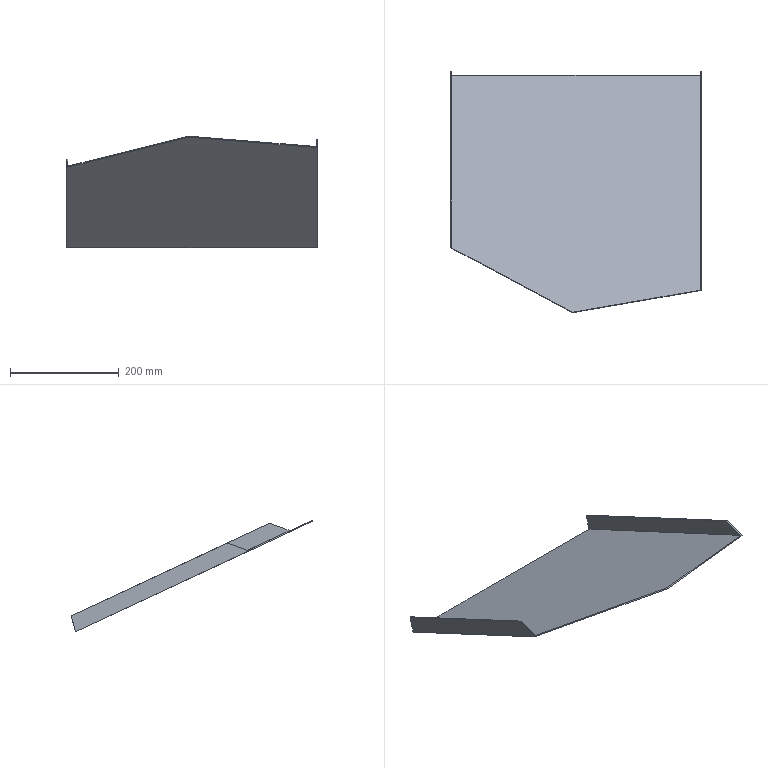Part | NX | features solid 2 | 1 solid | 13 faces | box 459.123 x 443.36 x 204.878 mm | volume 442508 mm3 | plane 12 | spline 1
STEP:
#1=CARTESIAN_POINT('',(40.63,399.571,-277.28));
#2=VERTEX_POINT('',#1);
#3=CARTESIAN_POINT('',(40.63,793.782,-461.104));
#4=VERTEX_POINT('',#3);
#5=CARTESIAN_POINT('',(40.63,358.626,-258.187));
#6=DIRECTION('',(0.,0.9063,-0.4226));
#7=VECTOR('',#6,1000.);
#8=LINE('',#5,#7);
#9=EDGE_CURVE('',#2,#4,#8,.T.);
#10=ORIENTED_EDGE('',*,*,#9,.T.);
#11=CARTESIAN_POINT('',(-414.493,793.782,-461.104));
#12=VERTEX_POINT('',#11);
#13=CARTESIAN_POINT('',(-192.912,793.782,-461.104));
#14=DIRECTION('',(-1.,0.,0.));
#15=VECTOR('',#14,1000.);
#16=LINE('',#13,#15);
#17=EDGE_CURVE('',#4,#12,#16,.T.);
#18=ORIENTED_EDGE('',*,*,#17,.T.);
#19=CARTESIAN_POINT('',(-414.493,477.671,-313.699));
#20=VERTEX_POINT('',#19);
#21=CARTESIAN_POINT('',(-414.493,358.626,-258.187));
#22=DIRECTION('',(0.,0.9063,-0.4226));
#23=VECTOR('',#22,1000.);
#24=LINE('',#21,#23);
#25=EDGE_CURVE('',#20,#12,#24,.T.);
#26=ORIENTED_EDGE('',*,*,#25,.F.);
#27=CARTESIAN_POINT('',(-416.493,477.671,-313.699));
#28=VERTEX_POINT('',#27);
#29=CARTESIAN_POINT('',(-416.493,477.671,-313.699));
#30=DIRECTION('',(-1.,0.,0.));
#31=VECTOR('',#30,1000.);
#32=LINE('',#29,#31);
#33=EDGE_CURVE('',#20,#28,#32,.T.);
#34=ORIENTED_EDGE('',*,*,#33,.T.);
#35=CARTESIAN_POINT('',(-192.912,358.626,-258.187));
#36=VERTEX_POINT('',#35);
#37=CARTESIAN_POINT('',(-192.912,358.626,-258.187));
#38=DIRECTION('',(0.8622,-0.4591,0.2141));
#39=VECTOR('',#38,1000.);
#40=LINE('',#37,#39);
#41=EDGE_CURVE('',#28,#36,#40,.T.);
#42=ORIENTED_EDGE('',*,*,#41,.T.);
#43=CARTESIAN_POINT('',(42.63,399.571,-277.28));
#44=VERTEX_POINT('',#43);
#45=CARTESIAN_POINT('',(-192.912,358.626,-258.187));
#46=CARTESIAN_POINT('',(-183.102,360.356,-258.994));
#47=CARTESIAN_POINT('',(-163.484,363.815,-260.607));
#48=CARTESIAN_POINT('',(-134.056,369.003,-263.026));
#49=CARTESIAN_POINT('',(-104.626,374.192,-265.446));
#50=CARTESIAN_POINT('',(-80.109,378.513,-267.461));
#51=CARTESIAN_POINT('',(-62.932,381.543,-268.874));
#52=CARTESIAN_POINT('',(-53.141,383.273,-269.68));
#53=CARTESIAN_POINT('',(-45.731,384.584,-270.292));
#54=CARTESIAN_POINT('',(-38.576,385.847,-270.88));
#55=CARTESIAN_POINT('',(-31.239,387.132,-271.48));
#56=CARTESIAN_POINT('',(-25.081,388.204,-271.98));
#57=CARTESIAN_POINT('',(-20.086,389.069,-272.383));
#58=CARTESIAN_POINT('',(-16.374,389.711,-272.682));
#59=CARTESIAN_POINT('',(-12.429,390.39,-272.999));
#60=CARTESIAN_POINT('',(-8.618,391.042,-273.303));
#61=CARTESIAN_POINT('',(-4.844,391.685,-273.603));
#62=CARTESIAN_POINT('',(-1.133,392.314,-273.896));
#63=CARTESIAN_POINT('',(2.523,392.93,-274.184));
#64=CARTESIAN_POINT('',(5.521,393.433,-274.418));
#65=CARTESIAN_POINT('',(7.891,393.829,-274.602));
#66=CARTESIAN_POINT('',(9.657,394.123,-274.74));
#67=CARTESIAN_POINT('',(11.104,394.363,-274.852));
#68=CARTESIAN_POINT('',(12.137,394.534,-274.931));
#69=CARTESIAN_POINT('',(12.684,394.624,-274.973));
#70=CARTESIAN_POINT('',(13.211,394.711,-275.014));
#71=CARTESIAN_POINT('',(13.289,394.724,-275.02));
#72=CARTESIAN_POINT('',(13.565,394.77,-275.041));
#73=CARTESIAN_POINT('',(14.006,394.843,-275.075));
#74=CARTESIAN_POINT('',(14.766,394.968,-275.134));
#75=CARTESIAN_POINT('',(15.806,395.14,-275.214));
#76=CARTESIAN_POINT('',(17.393,395.402,-275.336));
#77=CARTESIAN_POINT('',(19.737,395.789,-275.517));
#78=CARTESIAN_POINT('',(23.133,396.35,-275.778));
#79=CARTESIAN_POINT('',(27.111,397.007,-276.085));
#80=CARTESIAN_POINT('',(33.19,398.012,-276.553));
#81=CARTESIAN_POINT('',(38.621,398.909,-276.971));
#82=CARTESIAN_POINT('',(42.63,399.571,-277.28));
#83=B_SPLINE_CURVE_WITH_KNOTS('',3,(#45,#46,#47,#48,#49,#50,#51,#52,#53,#54,#55,#56,#57,#58,#59,#60,#61,#62,#63,#64,#65,#66,#67,#68,#69,#70,#71,#72,#73,#74,#75,#76,#77,#78,#79,#80,#81,#82),.UNSPECIFIED.,.F.,.F.,(4,1,1,1,1,1,1,1,1,1,1,1,1,1,1,1,1,1,1,1,1,1,1,1,1,1,1,1,1,1,1,1,1,1,1,4),(0.,0.125,0.25,0.375,0.5,0.5625,0.5938,0.625,0.6562,0.6875,0.7188,0.7344,0.75,0.7656,0.7812,0.7969,0.8125,0.8281,0.8438,0.8516,0.8594,0.8672,0.8711,0.873,0.875,0.877,0.8789,0.8828,0.8906,0.8984,0.9062,0.9219,0.9375,0.9531,0.9688,1.),.UNSPECIFIED.);
#84=EDGE_CURVE('',#44,#36,#83,.F.);
#85=ORIENTED_EDGE('',*,*,#84,.F.);
#86=CARTESIAN_POINT('',(42.63,399.571,-277.28));
#87=DIRECTION('',(1.,0.,0.));
#88=VECTOR('',#87,1000.);
#89=LINE('',#86,#88);
#90=EDGE_CURVE('',#44,#2,#89,.F.);
#91=ORIENTED_EDGE('',*,*,#90,.T.);
#92=EDGE_LOOP('',(#10,#18,#26,#34,#42,#85,#91));
#93=FACE_BOUND('',#92,.T.);
#94=CARTESIAN_POINT('',(-192.912,358.626,-258.187));
#95=DIRECTION('',(0.,-0.4226,-0.9063));
#96=DIRECTION('',(-1.,0.,0.));
#97=AXIS2_PLACEMENT_3D('',#94,#95,#96);
#98=PLANE('',#97);
#99=ADVANCED_FACE('',(#93),#98,.F.);
#100=ORIENTED_EDGE('',*,*,#84,.T.);
#101=CARTESIAN_POINT('',(-192.912,357.781,-260.));
#102=VERTEX_POINT('',#101);
#103=CARTESIAN_POINT('',(-192.912,358.626,-258.187));
#104=CARTESIAN_POINT('',(-192.912,358.345,-258.792));
#105=CARTESIAN_POINT('',(-192.912,358.063,-259.396));
#106=CARTESIAN_POINT('',(-192.912,357.781,-260.));
#107=B_SPLINE_CURVE_WITH_KNOTS('',3,(#103,#104,#105,#106),.UNSPECIFIED.,.F.,.F.,(4,4),(0.,1.),.UNSPECIFIED.);
#108=EDGE_CURVE('',#102,#36,#107,.F.);
#109=ORIENTED_EDGE('',*,*,#108,.F.);
#110=CARTESIAN_POINT('',(42.63,398.726,-279.093));
#111=VERTEX_POINT('',#110);
#112=CARTESIAN_POINT('',(-192.912,357.781,-260.));
#113=CARTESIAN_POINT('',(-183.102,359.511,-260.807));
#114=CARTESIAN_POINT('',(-163.484,362.97,-262.42));
#115=CARTESIAN_POINT('',(-134.056,368.158,-264.839));
#116=CARTESIAN_POINT('',(-104.626,373.347,-267.258));
#117=CARTESIAN_POINT('',(-80.109,377.668,-269.273));
#118=CARTESIAN_POINT('',(-62.932,380.698,-270.686));
#119=CARTESIAN_POINT('',(-53.141,382.427,-271.493));
#120=CARTESIAN_POINT('',(-45.731,383.739,-272.104));
#121=CARTESIAN_POINT('',(-38.576,385.001,-272.693));
#122=CARTESIAN_POINT('',(-31.239,386.287,-273.292));
#123=CARTESIAN_POINT('',(-25.081,387.359,-273.792));
#124=CARTESIAN_POINT('',(-20.086,388.224,-274.196));
#125=CARTESIAN_POINT('',(-16.374,388.865,-274.495));
#126=CARTESIAN_POINT('',(-12.429,389.544,-274.811));
#127=CARTESIAN_POINT('',(-8.618,390.197,-275.116));
#128=CARTESIAN_POINT('',(-4.844,390.84,-275.415));
#129=CARTESIAN_POINT('',(-1.133,391.469,-275.709));
#130=CARTESIAN_POINT('',(2.523,392.085,-275.996));
#131=CARTESIAN_POINT('',(5.521,392.588,-276.231));
#132=CARTESIAN_POINT('',(7.891,392.983,-276.415));
#133=CARTESIAN_POINT('',(9.657,393.277,-276.552));
#134=CARTESIAN_POINT('',(11.104,393.518,-276.664));
#135=CARTESIAN_POINT('',(12.137,393.689,-276.744));
#136=CARTESIAN_POINT('',(12.684,393.779,-276.786));
#137=CARTESIAN_POINT('',(13.211,393.866,-276.827));
#138=CARTESIAN_POINT('',(13.289,393.879,-276.833));
#139=CARTESIAN_POINT('',(13.565,393.925,-276.854));
#140=CARTESIAN_POINT('',(14.006,393.997,-276.888));
#141=CARTESIAN_POINT('',(14.766,394.123,-276.946));
#142=CARTESIAN_POINT('',(15.806,394.295,-277.027));
#143=CARTESIAN_POINT('',(17.393,394.557,-277.149));
#144=CARTESIAN_POINT('',(19.737,394.944,-277.329));
#145=CARTESIAN_POINT('',(23.133,395.505,-277.591));
#146=CARTESIAN_POINT('',(27.111,396.162,-277.897));
#147=CARTESIAN_POINT('',(33.19,397.166,-278.366));
#148=CARTESIAN_POINT('',(38.621,398.064,-278.784));
#149=CARTESIAN_POINT('',(42.63,398.726,-279.093));
#150=B_SPLINE_CURVE_WITH_KNOTS('',3,(#112,#113,#114,#115,#116,#117,#118,#119,#120,#121,#122,#123,#124,#125,#126,#127,#128,#129,#130,#131,#132,#133,#134,#135,#136,#137,#138,#139,#140,#141,#142,#143,#144,#145,#146,#147,#148,#149),.UNSPECIFIED.,.F.,.F.,(4,1,1,1,1,1,1,1,1,1,1,1,1,1,1,1,1,1,1,1,1,1,1,1,1,1,1,1,1,1,1,1,1,1,1,4),(0.,0.125,0.25,0.375,0.5,0.5625,0.5938,0.625,0.6562,0.6875,0.7188,0.7344,0.75,0.7656,0.7812,0.7969,0.8125,0.8281,0.8438,0.8516,0.8594,0.8672,0.8711,0.873,0.875,0.877,0.8789,0.8828,0.8906,0.8984,0.9062,0.9219,0.9375,0.9531,0.9688,1.),.UNSPECIFIED.);
#151=EDGE_CURVE('',#111,#102,#150,.F.);
#152=ORIENTED_EDGE('',*,*,#151,.F.);
#153=CARTESIAN_POINT('',(42.63,398.726,-279.093));
#154=CARTESIAN_POINT('',(42.63,399.008,-278.489));
#155=CARTESIAN_POINT('',(42.63,399.289,-277.884));
#156=CARTESIAN_POINT('',(42.63,399.571,-277.28));
#157=B_SPLINE_CURVE_WITH_KNOTS('',3,(#153,#154,#155,#156),.UNSPECIFIED.,.F.,.F.,(4,4),(0.,1.),.UNSPECIFIED.);
#158=EDGE_CURVE('',#111,#44,#157,.T.);
#159=ORIENTED_EDGE('',*,*,#158,.T.);
#160=EDGE_LOOP('',(#100,#109,#152,#159));
#161=FACE_BOUND('',#160,.T.);
#162=CARTESIAN_POINT('',(-192.912,357.781,-260.));
#163=CARTESIAN_POINT('',(-192.912,358.626,-258.187));
#164=CARTESIAN_POINT('',(-183.102,359.511,-260.807));
#165=CARTESIAN_POINT('',(-183.102,360.356,-258.994));
#166=CARTESIAN_POINT('',(-163.484,362.97,-262.42));
#167=CARTESIAN_POINT('',(-163.484,363.815,-260.607));
#168=CARTESIAN_POINT('',(-134.056,368.158,-264.839));
#169=CARTESIAN_POINT('',(-134.056,369.003,-263.026));
#170=CARTESIAN_POINT('',(-104.626,373.347,-267.258));
#171=CARTESIAN_POINT('',(-104.626,374.192,-265.446));
#172=CARTESIAN_POINT('',(-80.109,377.668,-269.273));
#173=CARTESIAN_POINT('',(-80.109,378.513,-267.461));
#174=CARTESIAN_POINT('',(-62.932,380.698,-270.686));
#175=CARTESIAN_POINT('',(-62.932,381.543,-268.874));
#176=CARTESIAN_POINT('',(-53.141,382.427,-271.493));
#177=CARTESIAN_POINT('',(-53.141,383.273,-269.68));
#178=CARTESIAN_POINT('',(-45.731,383.739,-272.104));
#179=CARTESIAN_POINT('',(-45.731,384.584,-270.292));
#180=CARTESIAN_POINT('',(-38.576,385.001,-272.693));
#181=CARTESIAN_POINT('',(-38.576,385.847,-270.88));
#182=CARTESIAN_POINT('',(-31.239,386.287,-273.292));
#183=CARTESIAN_POINT('',(-31.239,387.132,-271.48));
#184=CARTESIAN_POINT('',(-25.081,387.359,-273.792));
#185=CARTESIAN_POINT('',(-25.081,388.204,-271.98));
#186=CARTESIAN_POINT('',(-20.086,388.224,-274.196));
#187=CARTESIAN_POINT('',(-20.086,389.069,-272.383));
#188=CARTESIAN_POINT('',(-16.374,388.865,-274.495));
#189=CARTESIAN_POINT('',(-16.374,389.711,-272.682));
#190=CARTESIAN_POINT('',(-12.429,389.544,-274.811));
#191=CARTESIAN_POINT('',(-12.429,390.39,-272.999));
#192=CARTESIAN_POINT('',(-8.618,390.197,-275.116));
#193=CARTESIAN_POINT('',(-8.618,391.042,-273.303));
#194=CARTESIAN_POINT('',(-4.844,390.84,-275.415));
#195=CARTESIAN_POINT('',(-4.844,391.685,-273.603));
#196=CARTESIAN_POINT('',(-1.133,391.469,-275.709));
#197=CARTESIAN_POINT('',(-1.133,392.314,-273.896));
#198=CARTESIAN_POINT('',(2.523,392.085,-275.996));
#199=CARTESIAN_POINT('',(2.523,392.93,-274.184));
#200=CARTESIAN_POINT('',(5.521,392.588,-276.231));
#201=CARTESIAN_POINT('',(5.521,393.433,-274.418));
#202=CARTESIAN_POINT('',(7.891,392.983,-276.415));
#203=CARTESIAN_POINT('',(7.891,393.829,-274.602));
#204=CARTESIAN_POINT('',(9.657,393.277,-276.552));
#205=CARTESIAN_POINT('',(9.657,394.123,-274.74));
#206=CARTESIAN_POINT('',(11.104,393.518,-276.664));
#207=CARTESIAN_POINT('',(11.104,394.363,-274.852));
#208=CARTESIAN_POINT('',(12.137,393.689,-276.744));
#209=CARTESIAN_POINT('',(12.137,394.534,-274.931));
#210=CARTESIAN_POINT('',(12.684,393.779,-276.786));
#211=CARTESIAN_POINT('',(12.684,394.624,-274.973));
#212=CARTESIAN_POINT('',(13.211,393.866,-276.827));
#213=CARTESIAN_POINT('',(13.211,394.711,-275.014));
#214=CARTESIAN_POINT('',(13.289,393.879,-276.833));
#215=CARTESIAN_POINT('',(13.289,394.724,-275.02));
#216=CARTESIAN_POINT('',(13.565,393.925,-276.854));
#217=CARTESIAN_POINT('',(13.565,394.77,-275.041));
#218=CARTESIAN_POINT('',(14.006,393.997,-276.888));
#219=CARTESIAN_POINT('',(14.006,394.843,-275.075));
#220=CARTESIAN_POINT('',(14.766,394.123,-276.946));
#221=CARTESIAN_POINT('',(14.766,394.968,-275.134));
#222=CARTESIAN_POINT('',(15.806,394.295,-277.027));
#223=CARTESIAN_POINT('',(15.806,395.14,-275.214));
#224=CARTESIAN_POINT('',(17.393,394.557,-277.149));
#225=CARTESIAN_POINT('',(17.393,395.402,-275.336));
#226=CARTESIAN_POINT('',(19.737,394.944,-277.329));
#227=CARTESIAN_POINT('',(19.737,395.789,-275.517));
#228=CARTESIAN_POINT('',(23.133,395.505,-277.591));
#229=CARTESIAN_POINT('',(23.133,396.35,-275.778));
#230=CARTESIAN_POINT('',(27.111,396.162,-277.897));
#231=CARTESIAN_POINT('',(27.111,397.007,-276.085));
#232=CARTESIAN_POINT('',(33.19,397.166,-278.366));
#233=CARTESIAN_POINT('',(33.19,398.012,-276.553));
#234=CARTESIAN_POINT('',(38.621,398.064,-278.784));
#235=CARTESIAN_POINT('',(38.621,398.909,-276.971));
#236=CARTESIAN_POINT('',(42.63,398.726,-279.093));
#237=CARTESIAN_POINT('',(42.63,399.571,-277.28));
#238=B_SPLINE_SURFACE_WITH_KNOTS('',3,1,((#162,#163),(#164,#165),(#166,#167),(#168,#169),(#170,#171),(#172,#173),(#174,#175),(#176,#177),(#178,#179),(#180,#181),(#182,#183),(#184,#185),(#186,#187),(#188,#189),(#190,#191),(#192,#193),(#194,#195),(#196,#197),(#198,#199),(#200,#201),(#202,#203),(#204,#205),(#206,#207),(#208,#209),(#210,#211),(#212,#213),(#214,#215),(#216,#217),(#218,#219),(#220,#221),(#222,#223),(#224,#225),(#226,#227),(#228,#229),(#230,#231),(#232,#233),(#234,#235),(#236,#237)),.SURF_OF_LINEAR_EXTRUSION.,.F.,.F.,.F.,(4,1,1,1,1,1,1,1,1,1,1,1,1,1,1,1,1,1,1,1,1,1,1,1,1,1,1,1,1,1,1,1,1,1,1,4),(2,2),(0.,0.125,0.25,0.375,0.5,0.5625,0.5938,0.625,0.6562,0.6875,0.7188,0.7344,0.75,0.7656,0.7812,0.7969,0.8125,0.8281,0.8438,0.8516,0.8594,0.8672,0.8711,0.873,0.875,0.877,0.8789,0.8828,0.8906,0.8984,0.9062,0.9219,0.9375,0.9531,0.9688,1.),(0.,1.),.UNSPECIFIED.);
#239=ADVANCED_FACE('',(#161),#238,.T.);
#240=CARTESIAN_POINT('',(42.63,793.257,-463.066));
#241=VERTEX_POINT('',#240);
#242=CARTESIAN_POINT('',(42.63,357.781,-260.));
#243=DIRECTION('',(0.,-0.9063,0.4226));
#244=VECTOR('',#243,1000.);
#245=LINE('',#242,#244);
#246=EDGE_CURVE('',#241,#111,#245,.T.);
#247=ORIENTED_EDGE('',*,*,#246,.F.);
#248=CARTESIAN_POINT('',(42.63,801.141,-433.641));
#249=VERTEX_POINT('',#248);
#250=CARTESIAN_POINT('',(42.63,814.852,-382.472));
#251=DIRECTION('',(0.,0.2588,0.9659));
#252=VECTOR('',#251,1000.);
#253=LINE('',#250,#252);
#254=EDGE_CURVE('',#241,#249,#253,.T.);
#255=ORIENTED_EDGE('',*,*,#254,.T.);
#256=CARTESIAN_POINT('',(42.63,436.781,-263.737));
#257=VERTEX_POINT('',#256);
#258=CARTESIAN_POINT('',(42.63,1052.679,-550.935));
#259=DIRECTION('',(0.,-0.9063,0.4226));
#260=VECTOR('',#259,1000.);
#261=LINE('',#258,#260);
#262=EDGE_CURVE('',#249,#257,#261,.T.);
#263=ORIENTED_EDGE('',*,*,#262,.T.);
#264=CARTESIAN_POINT('',(42.63,399.571,-277.28));
#265=DIRECTION('',(0.,-0.9397,-0.342));
#266=VECTOR('',#265,1000.);
#267=LINE('',#264,#266);
#268=EDGE_CURVE('',#257,#44,#267,.T.);
#269=ORIENTED_EDGE('',*,*,#268,.T.);
#270=ORIENTED_EDGE('',*,*,#158,.F.);
#271=EDGE_LOOP('',(#247,#255,#263,#269,#270));
#272=FACE_BOUND('',#271,.T.);
#273=CARTESIAN_POINT('',(42.63,357.781,-260.));
#274=DIRECTION('',(-1.,0.,0.));
#275=DIRECTION('',(0.,0.,1.));
#276=AXIS2_PLACEMENT_3D('',#273,#274,#275);
#277=PLANE('',#276);
#278=ADVANCED_FACE('',(#272),#277,.F.);
#279=CARTESIAN_POINT('',(-416.493,793.257,-463.066));
#280=VERTEX_POINT('',#279);
#281=CARTESIAN_POINT('',(-416.493,801.141,-433.641));
#282=VERTEX_POINT('',#281);
#283=CARTESIAN_POINT('',(-416.493,814.852,-382.472));
#284=DIRECTION('',(0.,0.2588,0.9659));
#285=VECTOR('',#284,1000.);
#286=LINE('',#283,#285);
#287=EDGE_CURVE('',#280,#282,#286,.T.);
#288=ORIENTED_EDGE('',*,*,#287,.F.);
#289=CARTESIAN_POINT('',(-416.493,476.826,-315.512));
#290=VERTEX_POINT('',#289);
#291=CARTESIAN_POINT('',(-416.493,357.781,-260.));
#292=DIRECTION('',(0.,-0.9063,0.4226));
#293=VECTOR('',#292,1000.);
#294=LINE('',#291,#293);
#295=EDGE_CURVE('',#280,#290,#294,.T.);
#296=ORIENTED_EDGE('',*,*,#295,.T.);
#297=CARTESIAN_POINT('',(-416.493,476.826,-315.512));
#298=DIRECTION('',(0.,0.4226,0.9063));
#299=VECTOR('',#298,1000.);
#300=LINE('',#297,#299);
#301=EDGE_CURVE('',#290,#28,#300,.T.);
#302=ORIENTED_EDGE('',*,*,#301,.T.);
#303=CARTESIAN_POINT('',(-416.493,514.881,-300.156));
#304=VERTEX_POINT('',#303);
#305=CARTESIAN_POINT('',(-416.493,889.235,-163.902));
#306=DIRECTION('',(0.,0.9397,0.342));
#307=VECTOR('',#306,1000.);
#308=LINE('',#305,#307);
#309=EDGE_CURVE('',#28,#304,#308,.T.);
#310=ORIENTED_EDGE('',*,*,#309,.T.);
#311=CARTESIAN_POINT('',(-416.493,1052.679,-550.935));
#312=DIRECTION('',(0.,-0.9063,0.4226));
#313=VECTOR('',#312,1000.);
#314=LINE('',#311,#313);
#315=EDGE_CURVE('',#282,#304,#314,.T.);
#316=ORIENTED_EDGE('',*,*,#315,.F.);
#317=EDGE_LOOP('',(#288,#296,#302,#310,#316));
#318=FACE_BOUND('',#317,.T.);
#319=CARTESIAN_POINT('',(-416.493,357.781,-260.));
#320=DIRECTION('',(-1.,0.,0.));
#321=DIRECTION('',(0.,0.,1.));
#322=AXIS2_PLACEMENT_3D('',#319,#320,#321);
#323=PLANE('',#322);
#324=ADVANCED_FACE('',(#318),#323,.T.);
#325=ORIENTED_EDGE('',*,*,#41,.F.);
#326=ORIENTED_EDGE('',*,*,#301,.F.);
#327=CARTESIAN_POINT('',(-192.912,357.781,-260.));
#328=DIRECTION('',(0.8622,-0.4591,0.2141));
#329=VECTOR('',#328,1000.);
#330=LINE('',#327,#329);
#331=EDGE_CURVE('',#290,#102,#330,.T.);
#332=ORIENTED_EDGE('',*,*,#331,.T.);
#333=ORIENTED_EDGE('',*,*,#108,.T.);
#334=EDGE_LOOP('',(#325,#326,#332,#333));
#335=FACE_BOUND('',#334,.T.);
#336=CARTESIAN_POINT('',(-192.912,357.781,-260.));
#337=DIRECTION('',(-0.5065,-0.7814,0.3644));
#338=DIRECTION('',(0.8391,-0.5439,0.));
#339=AXIS2_PLACEMENT_3D('',#336,#337,#338);
#340=PLANE('',#339);
#341=ADVANCED_FACE('',(#335),#340,.T.);
#342=CARTESIAN_POINT('',(-192.912,793.257,-463.066));
#343=DIRECTION('',(-1.,0.,0.));
#344=VECTOR('',#343,1000.);
#345=LINE('',#342,#344);
#346=EDGE_CURVE('',#241,#280,#345,.T.);
#347=ORIENTED_EDGE('',*,*,#346,.F.);
#348=ORIENTED_EDGE('',*,*,#246,.T.);
#349=ORIENTED_EDGE('',*,*,#151,.T.);
#350=ORIENTED_EDGE('',*,*,#331,.F.);
#351=ORIENTED_EDGE('',*,*,#295,.F.);
#352=EDGE_LOOP('',(#347,#348,#349,#350,#351));
#353=FACE_BOUND('',#352,.T.);
#354=CARTESIAN_POINT('',(-192.912,357.781,-260.));
#355=DIRECTION('',(0.,-0.4226,-0.9063));
#356=DIRECTION('',(-1.,0.,0.));
#357=AXIS2_PLACEMENT_3D('',#354,#355,#356);
#358=PLANE('',#357);
#359=ADVANCED_FACE('',(#353),#358,.T.);
#360=ORIENTED_EDGE('',*,*,#262,.F.);
#361=CARTESIAN_POINT('',(40.63,801.141,-433.641));
#362=VERTEX_POINT('',#361);
#363=CARTESIAN_POINT('',(42.63,801.141,-433.641));
#364=DIRECTION('',(-1.,0.,0.));
#365=VECTOR('',#364,1000.);
#366=LINE('',#363,#365);
#367=EDGE_CURVE('',#249,#362,#366,.T.);
#368=ORIENTED_EDGE('',*,*,#367,.T.);
#369=CARTESIAN_POINT('',(40.63,436.781,-263.737));
#370=VERTEX_POINT('',#369);
#371=CARTESIAN_POINT('',(40.63,1052.679,-550.935));
#372=DIRECTION('',(0.,-0.9063,0.4226));
#373=VECTOR('',#372,1000.);
#374=LINE('',#371,#373);
#375=EDGE_CURVE('',#362,#370,#374,.T.);
#376=ORIENTED_EDGE('',*,*,#375,.T.);
#377=CARTESIAN_POINT('',(42.63,436.781,-263.737));
#378=DIRECTION('',(1.,0.,0.));
#379=VECTOR('',#378,1000.);
#380=LINE('',#377,#379);
#381=EDGE_CURVE('',#370,#257,#380,.T.);
#382=ORIENTED_EDGE('',*,*,#381,.T.);
#383=EDGE_LOOP('',(#360,#368,#376,#382));
#384=FACE_BOUND('',#383,.T.);
#385=CARTESIAN_POINT('',(42.63,1052.679,-550.935));
#386=DIRECTION('',(0.,-0.4226,-0.9063));
#387=DIRECTION('',(0.,-0.9063,0.4226));
#388=AXIS2_PLACEMENT_3D('',#385,#386,#387);
#389=PLANE('',#388);
#390=ADVANCED_FACE('',(#384),#389,.F.);
#391=CARTESIAN_POINT('',(40.63,781.021,-508.731));
#392=DIRECTION('',(0.,0.2588,0.9659));
#393=VECTOR('',#392,1000.);
#394=LINE('',#391,#393);
#395=EDGE_CURVE('',#4,#362,#394,.T.);
#396=ORIENTED_EDGE('',*,*,#395,.F.);
#397=ORIENTED_EDGE('',*,*,#9,.F.);
#398=CARTESIAN_POINT('',(40.63,868.395,-106.642));
#399=DIRECTION('',(0.,0.9397,0.342));
#400=VECTOR('',#399,1000.);
#401=LINE('',#398,#400);
#402=EDGE_CURVE('',#2,#370,#401,.T.);
#403=ORIENTED_EDGE('',*,*,#402,.T.);
#404=ORIENTED_EDGE('',*,*,#375,.F.);
#405=EDGE_LOOP('',(#396,#397,#403,#404));
#406=FACE_BOUND('',#405,.T.);
#407=CARTESIAN_POINT('',(40.63,1040.,-578.124));
#408=DIRECTION('',(-1.,0.,0.));
#409=DIRECTION('',(0.,0.,1.));
#410=AXIS2_PLACEMENT_3D('',#407,#408,#409);
#411=PLANE('',#410);
#412=ADVANCED_FACE('',(#406),#411,.T.);
#413=ORIENTED_EDGE('',*,*,#268,.F.);
#414=ORIENTED_EDGE('',*,*,#381,.F.);
#415=ORIENTED_EDGE('',*,*,#402,.F.);
#416=ORIENTED_EDGE('',*,*,#90,.F.);
#417=EDGE_LOOP('',(#413,#414,#415,#416));
#418=FACE_BOUND('',#417,.T.);
#419=CARTESIAN_POINT('',(42.63,399.571,-277.28));
#420=DIRECTION('',(0.,-0.342,0.9397));
#421=DIRECTION('',(0.,-0.9397,-0.342));
#422=AXIS2_PLACEMENT_3D('',#419,#420,#421);
#423=PLANE('',#422);
#424=ADVANCED_FACE('',(#418),#423,.T.);
#425=CARTESIAN_POINT('',(-414.493,801.141,-433.641));
#426=VERTEX_POINT('',#425);
#427=CARTESIAN_POINT('',(-416.493,801.141,-433.641));
#428=DIRECTION('',(-1.,0.,0.));
#429=VECTOR('',#428,1000.);
#430=LINE('',#427,#429);
#431=EDGE_CURVE('',#282,#426,#430,.F.);
#432=ORIENTED_EDGE('',*,*,#431,.F.);
#433=ORIENTED_EDGE('',*,*,#315,.T.);
#434=CARTESIAN_POINT('',(-414.493,514.881,-300.156));
#435=VERTEX_POINT('',#434);
#436=CARTESIAN_POINT('',(-416.493,514.881,-300.156));
#437=DIRECTION('',(-1.,0.,0.));
#438=VECTOR('',#437,1000.);
#439=LINE('',#436,#438);
#440=EDGE_CURVE('',#304,#435,#439,.F.);
#441=ORIENTED_EDGE('',*,*,#440,.T.);
#442=CARTESIAN_POINT('',(-414.493,1052.679,-550.935));
#443=DIRECTION('',(0.,-0.9063,0.4226));
#444=VECTOR('',#443,1000.);
#445=LINE('',#442,#444);
#446=EDGE_CURVE('',#426,#435,#445,.T.);
#447=ORIENTED_EDGE('',*,*,#446,.F.);
#448=EDGE_LOOP('',(#432,#433,#441,#447));
#449=FACE_BOUND('',#448,.T.);
#450=CARTESIAN_POINT('',(-416.493,1052.679,-550.935));
#451=DIRECTION('',(0.,-0.4226,-0.9063));
#452=DIRECTION('',(0.,-0.9063,0.4226));
#453=AXIS2_PLACEMENT_3D('',#450,#451,#452);
#454=PLANE('',#453);
#455=ADVANCED_FACE('',(#449),#454,.F.);
#456=ORIENTED_EDGE('',*,*,#25,.T.);
#457=CARTESIAN_POINT('',(-414.493,781.021,-508.731));
#458=DIRECTION('',(0.,0.2588,0.9659));
#459=VECTOR('',#458,1000.);
#460=LINE('',#457,#459);
#461=EDGE_CURVE('',#12,#426,#460,.T.);
#462=ORIENTED_EDGE('',*,*,#461,.T.);
#463=ORIENTED_EDGE('',*,*,#446,.T.);
#464=CARTESIAN_POINT('',(-414.493,514.881,-300.156));
#465=DIRECTION('',(0.,-0.9397,-0.342));
#466=VECTOR('',#465,1000.);
#467=LINE('',#464,#466);
#468=EDGE_CURVE('',#435,#20,#467,.T.);
#469=ORIENTED_EDGE('',*,*,#468,.T.);
#470=EDGE_LOOP('',(#456,#462,#463,#469));
#471=FACE_BOUND('',#470,.T.);
#472=CARTESIAN_POINT('',(-414.493,1040.,-578.124));
#473=DIRECTION('',(-1.,0.,0.));
#474=DIRECTION('',(0.,0.,1.));
#475=AXIS2_PLACEMENT_3D('',#472,#473,#474);
#476=PLANE('',#475);
#477=ADVANCED_FACE('',(#471),#476,.F.);
#478=ORIENTED_EDGE('',*,*,#309,.F.);
#479=ORIENTED_EDGE('',*,*,#33,.F.);
#480=ORIENTED_EDGE('',*,*,#468,.F.);
#481=ORIENTED_EDGE('',*,*,#440,.F.);
#482=EDGE_LOOP('',(#478,#479,#480,#481));
#483=FACE_BOUND('',#482,.T.);
#484=CARTESIAN_POINT('',(-416.493,514.881,-300.156));
#485=DIRECTION('',(0.,-0.342,0.9397));
#486=DIRECTION('',(0.,-0.9397,-0.342));
#487=AXIS2_PLACEMENT_3D('',#484,#485,#486);
#488=PLANE('',#487);
#489=ADVANCED_FACE('',(#483),#488,.T.);
#490=ORIENTED_EDGE('',*,*,#254,.F.);
#491=ORIENTED_EDGE('',*,*,#346,.T.);
#492=ORIENTED_EDGE('',*,*,#287,.T.);
#493=ORIENTED_EDGE('',*,*,#431,.T.);
#494=ORIENTED_EDGE('',*,*,#461,.F.);
#495=ORIENTED_EDGE('',*,*,#17,.F.);
#496=ORIENTED_EDGE('',*,*,#395,.T.);
#497=ORIENTED_EDGE('',*,*,#367,.F.);
#498=EDGE_LOOP('',(#490,#491,#492,#493,#494,#495,#496,#497));
#499=FACE_BOUND('',#498,.T.);
#500=CARTESIAN_POINT('',(-426.493,792.089,-467.423));
#501=DIRECTION('',(0.,-0.9659,0.2588));
#502=DIRECTION('',(0.,-0.2588,-0.9659));
#503=AXIS2_PLACEMENT_3D('',#500,#501,#502);
#504=PLANE('',#503);
#505=ADVANCED_FACE('',(#499),#504,.F.);
#506=CLOSED_SHELL('',(#99,#239,#278,#324,#341,#359,#390,#412,#424,#455,#477,#489,#505));
#507=MANIFOLD_SOLID_BREP('',#506);
#508=(LENGTH_UNIT()NAMED_UNIT(*)SI_UNIT(.MILLI.,.METRE.));
#509=UNCERTAINTY_MEASURE_WITH_UNIT(LENGTH_MEASURE(0.0508),#508,'','');
#510=(NAMED_UNIT(*)PLANE_ANGLE_UNIT()SI_UNIT($,.RADIAN.));
#511=(NAMED_UNIT(*)SI_UNIT($,.STERADIAN.)SOLID_ANGLE_UNIT());
#512=(GEOMETRIC_REPRESENTATION_CONTEXT(3)GLOBAL_UNCERTAINTY_ASSIGNED_CONTEXT((#509))GLOBAL_UNIT_ASSIGNED_CONTEXT((#508,#510,#511))REPRESENTATION_CONTEXT('',''));
#513=ADVANCED_BREP_SHAPE_REPRESENTATION('',(#507),#512);